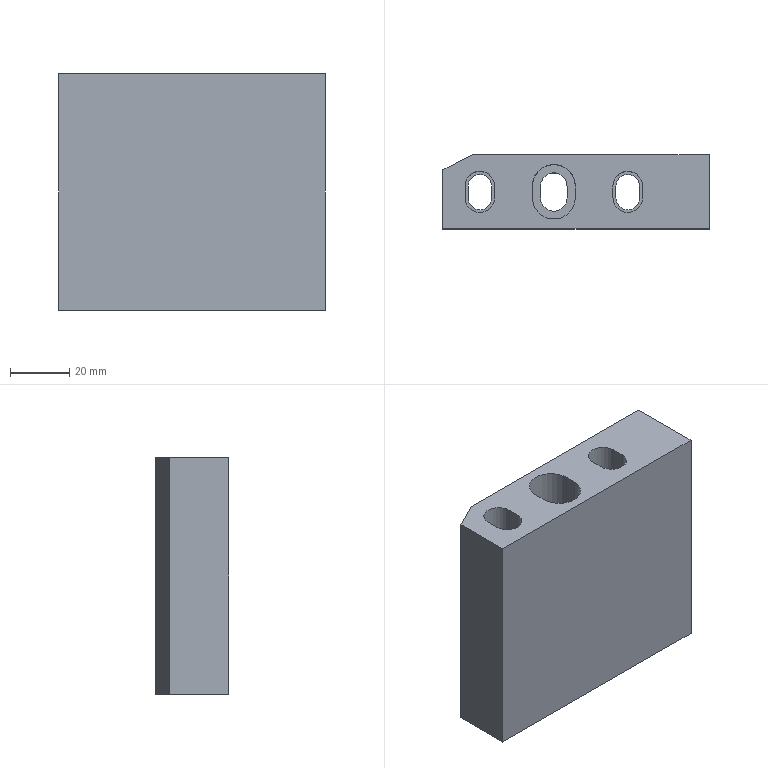Part | STEP file | 1 solid | 34 faces | box 90 x 25 x 80 mm | volume 146448 mm3 | plane 22 | cylinder 12 | commonest cylinder face diameters 8 x4 10 x4 9 x2 14.5 x2
STEP:
#1=CARTESIAN_POINT('',(257.5,-111.,33.));
#2=VERTEX_POINT('',#1);
#3=CARTESIAN_POINT('',(247.5,-111.,33.));
#4=VERTEX_POINT('',#3);
#5=CARTESIAN_POINT('',(252.5,-111.,33.));
#6=DIRECTION('',(0.,0.,-1.));
#7=DIRECTION('',(1.,0.,0.));
#8=AXIS2_PLACEMENT_3D('',#5,#6,#7);
#9=CIRCLE('',#8,5.);
#10=EDGE_CURVE('',#2,#4,#9,.T.);
#11=ORIENTED_EDGE('',*,*,#10,.T.);
#12=CARTESIAN_POINT('',(247.5,-107.,33.));
#13=VERTEX_POINT('',#12);
#14=CARTESIAN_POINT('',(247.5,3.,33.));
#15=DIRECTION('',(0.,1.,0.));
#16=VECTOR('',#15,1.);
#17=LINE('',#14,#16);
#18=EDGE_CURVE('',#4,#13,#17,.T.);
#19=ORIENTED_EDGE('',*,*,#18,.T.);
#20=CARTESIAN_POINT('',(257.5,-107.,33.));
#21=VERTEX_POINT('',#20);
#22=CARTESIAN_POINT('',(252.5,-107.,33.));
#23=DIRECTION('',(0.,0.,-1.));
#24=DIRECTION('',(1.,0.,0.));
#25=AXIS2_PLACEMENT_3D('',#22,#23,#24);
#26=CIRCLE('',#25,5.);
#27=EDGE_CURVE('',#13,#21,#26,.T.);
#28=ORIENTED_EDGE('',*,*,#27,.T.);
#29=CARTESIAN_POINT('',(257.5,3.,33.));
#30=DIRECTION('',(0.,1.,0.));
#31=VECTOR('',#30,1.);
#32=LINE('',#29,#31);
#33=EDGE_CURVE('',#2,#21,#32,.T.);
#34=ORIENTED_EDGE('',*,*,#33,.F.);
#35=EDGE_LOOP('',(#11,#19,#28,#34));
#36=FACE_BOUND('',#35,.T.);
#37=CARTESIAN_POINT('',(307.5,-111.,33.));
#38=VERTEX_POINT('',#37);
#39=CARTESIAN_POINT('',(297.5,-111.,33.));
#40=VERTEX_POINT('',#39);
#41=CARTESIAN_POINT('',(302.5,-111.,33.));
#42=DIRECTION('',(0.,0.,-1.));
#43=DIRECTION('',(1.,0.,0.));
#44=AXIS2_PLACEMENT_3D('',#41,#42,#43);
#45=CIRCLE('',#44,5.);
#46=EDGE_CURVE('',#38,#40,#45,.T.);
#47=ORIENTED_EDGE('',*,*,#46,.T.);
#48=CARTESIAN_POINT('',(297.5,-107.,33.));
#49=VERTEX_POINT('',#48);
#50=CARTESIAN_POINT('',(297.5,3.,33.));
#51=DIRECTION('',(0.,1.,0.));
#52=VECTOR('',#51,1.);
#53=LINE('',#50,#52);
#54=EDGE_CURVE('',#40,#49,#53,.T.);
#55=ORIENTED_EDGE('',*,*,#54,.T.);
#56=CARTESIAN_POINT('',(307.5,-107.,33.));
#57=VERTEX_POINT('',#56);
#58=CARTESIAN_POINT('',(302.5,-107.,33.));
#59=DIRECTION('',(0.,0.,-1.));
#60=DIRECTION('',(1.,0.,0.));
#61=AXIS2_PLACEMENT_3D('',#58,#59,#60);
#62=CIRCLE('',#61,5.);
#63=EDGE_CURVE('',#49,#57,#62,.T.);
#64=ORIENTED_EDGE('',*,*,#63,.T.);
#65=CARTESIAN_POINT('',(307.5,3.,33.));
#66=DIRECTION('',(0.,1.,0.));
#67=VECTOR('',#66,1.);
#68=LINE('',#65,#67);
#69=EDGE_CURVE('',#38,#57,#68,.T.);
#70=ORIENTED_EDGE('',*,*,#69,.F.);
#71=EDGE_LOOP('',(#47,#55,#64,#70));
#72=FACE_BOUND('',#71,.T.);
#73=CARTESIAN_POINT('',(284.75,-111.,33.));
#74=VERTEX_POINT('',#73);
#75=CARTESIAN_POINT('',(270.25,-111.,33.));
#76=VERTEX_POINT('',#75);
#77=CARTESIAN_POINT('',(277.5,-111.,33.));
#78=DIRECTION('',(0.,0.,-1.));
#79=DIRECTION('',(1.,0.,0.));
#80=AXIS2_PLACEMENT_3D('',#77,#78,#79);
#81=CIRCLE('',#80,7.25);
#82=EDGE_CURVE('',#74,#76,#81,.T.);
#83=ORIENTED_EDGE('',*,*,#82,.T.);
#84=CARTESIAN_POINT('',(270.25,-107.,33.));
#85=VERTEX_POINT('',#84);
#86=CARTESIAN_POINT('',(270.25,3.,33.));
#87=DIRECTION('',(0.,1.,0.));
#88=VECTOR('',#87,1.);
#89=LINE('',#86,#88);
#90=EDGE_CURVE('',#76,#85,#89,.T.);
#91=ORIENTED_EDGE('',*,*,#90,.T.);
#92=CARTESIAN_POINT('',(284.75,-107.,33.));
#93=VERTEX_POINT('',#92);
#94=CARTESIAN_POINT('',(277.5,-107.,33.));
#95=DIRECTION('',(0.,0.,-1.));
#96=DIRECTION('',(1.,0.,0.));
#97=AXIS2_PLACEMENT_3D('',#94,#95,#96);
#98=CIRCLE('',#97,7.25);
#99=EDGE_CURVE('',#85,#93,#98,.T.);
#100=ORIENTED_EDGE('',*,*,#99,.T.);
#101=CARTESIAN_POINT('',(284.75,3.,33.));
#102=DIRECTION('',(0.,1.,0.));
#103=VECTOR('',#102,1.);
#104=LINE('',#101,#103);
#105=EDGE_CURVE('',#74,#93,#104,.T.);
#106=ORIENTED_EDGE('',*,*,#105,.F.);
#107=EDGE_LOOP('',(#83,#91,#100,#106));
#108=FACE_BOUND('',#107,.T.);
#109=CARTESIAN_POINT('',(330.,-96.5,33.));
#110=VERTEX_POINT('',#109);
#111=CARTESIAN_POINT('',(250.,-96.5,33.));
#112=VERTEX_POINT('',#111);
#113=CARTESIAN_POINT('',(259.,-96.5,33.));
#114=DIRECTION('',(-1.,0.,0.));
#115=VECTOR('',#114,1.);
#116=LINE('',#113,#115);
#117=EDGE_CURVE('',#110,#112,#116,.T.);
#118=ORIENTED_EDGE('',*,*,#117,.T.);
#119=CARTESIAN_POINT('',(240.,-101.5,33.));
#120=VERTEX_POINT('',#119);
#121=CARTESIAN_POINT('',(240.,-101.5,33.));
#122=DIRECTION('',(-0.8944,-0.4472,0.));
#123=VECTOR('',#122,1.);
#124=LINE('',#121,#123);
#125=EDGE_CURVE('',#112,#120,#124,.T.);
#126=ORIENTED_EDGE('',*,*,#125,.T.);
#127=CARTESIAN_POINT('',(240.,-121.5,33.));
#128=VERTEX_POINT('',#127);
#129=CARTESIAN_POINT('',(240.,-74.5,33.));
#130=DIRECTION('',(0.,1.,0.));
#131=VECTOR('',#130,1.);
#132=LINE('',#129,#131);
#133=EDGE_CURVE('',#128,#120,#132,.T.);
#134=ORIENTED_EDGE('',*,*,#133,.F.);
#135=CARTESIAN_POINT('',(330.,-121.5,33.));
#136=VERTEX_POINT('',#135);
#137=CARTESIAN_POINT('',(259.,-121.5,33.));
#138=DIRECTION('',(-1.,0.,0.));
#139=VECTOR('',#138,1.);
#140=LINE('',#137,#139);
#141=EDGE_CURVE('',#136,#128,#140,.T.);
#142=ORIENTED_EDGE('',*,*,#141,.F.);
#143=CARTESIAN_POINT('',(330.,3.,33.));
#144=DIRECTION('',(0.,1.,0.));
#145=VECTOR('',#144,1.);
#146=LINE('',#143,#145);
#147=EDGE_CURVE('',#136,#110,#146,.T.);
#148=ORIENTED_EDGE('',*,*,#147,.T.);
#149=EDGE_LOOP('',(#118,#126,#134,#142,#148));
#150=FACE_BOUND('',#149,.T.);
#151=CARTESIAN_POINT('',(88.5,3.,33.));
#152=DIRECTION('',(0.,0.,1.));
#153=DIRECTION('',(1.,0.,0.));
#154=AXIS2_PLACEMENT_3D('',#151,#152,#153);
#155=PLANE('',#154);
#156=ADVANCED_FACE('',(#36,#72,#108,#150),#155,.T.);
#157=ORIENTED_EDGE('',*,*,#133,.T.);
#158=CARTESIAN_POINT('',(240.,-101.5,-47.));
#159=VERTEX_POINT('',#158);
#160=CARTESIAN_POINT('',(240.,-101.5,-47.));
#161=DIRECTION('',(0.,0.,-1.));
#162=VECTOR('',#161,1.);
#163=LINE('',#160,#162);
#164=EDGE_CURVE('',#120,#159,#163,.T.);
#165=ORIENTED_EDGE('',*,*,#164,.T.);
#166=CARTESIAN_POINT('',(240.,-121.5,-47.));
#167=VERTEX_POINT('',#166);
#168=CARTESIAN_POINT('',(240.,-74.5,-47.));
#169=DIRECTION('',(0.,1.,0.));
#170=VECTOR('',#169,1.);
#171=LINE('',#168,#170);
#172=EDGE_CURVE('',#167,#159,#171,.T.);
#173=ORIENTED_EDGE('',*,*,#172,.F.);
#174=CARTESIAN_POINT('',(240.,-121.5,-29.347));
#175=DIRECTION('',(0.,0.,-1.));
#176=VECTOR('',#175,1.);
#177=LINE('',#174,#176);
#178=EDGE_CURVE('',#128,#167,#177,.T.);
#179=ORIENTED_EDGE('',*,*,#178,.F.);
#180=EDGE_LOOP('',(#157,#165,#173,#179));
#181=FACE_OUTER_BOUND('',#180,.T.);
#182=CARTESIAN_POINT('',(240.,-74.5,-22.));
#183=DIRECTION('',(1.,0.,0.));
#184=DIRECTION('',(0.,0.,-1.));
#185=AXIS2_PLACEMENT_3D('',#182,#183,#184);
#186=PLANE('',#185);
#187=ADVANCED_FACE('',(#181),#186,.F.);
#188=CARTESIAN_POINT('',(256.5,-107.,-47.));
#189=VERTEX_POINT('',#188);
#190=CARTESIAN_POINT('',(248.5,-107.,-47.));
#191=VERTEX_POINT('',#190);
#192=CARTESIAN_POINT('',(252.5,-107.,-47.));
#193=DIRECTION('',(0.,0.,1.));
#194=DIRECTION('',(1.,0.,0.));
#195=AXIS2_PLACEMENT_3D('',#192,#193,#194);
#196=CIRCLE('',#195,4.);
#197=EDGE_CURVE('',#189,#191,#196,.T.);
#198=ORIENTED_EDGE('',*,*,#197,.T.);
#199=CARTESIAN_POINT('',(248.5,-111.,-47.));
#200=VERTEX_POINT('',#199);
#201=CARTESIAN_POINT('',(248.5,-74.5,-47.));
#202=DIRECTION('',(0.,-1.,0.));
#203=VECTOR('',#202,1.);
#204=LINE('',#201,#203);
#205=EDGE_CURVE('',#191,#200,#204,.T.);
#206=ORIENTED_EDGE('',*,*,#205,.T.);
#207=CARTESIAN_POINT('',(256.5,-111.,-47.));
#208=VERTEX_POINT('',#207);
#209=CARTESIAN_POINT('',(252.5,-111.,-47.));
#210=DIRECTION('',(0.,0.,1.));
#211=DIRECTION('',(1.,0.,0.));
#212=AXIS2_PLACEMENT_3D('',#209,#210,#211);
#213=CIRCLE('',#212,4.);
#214=EDGE_CURVE('',#200,#208,#213,.T.);
#215=ORIENTED_EDGE('',*,*,#214,.T.);
#216=CARTESIAN_POINT('',(256.5,-74.5,-47.));
#217=DIRECTION('',(0.,-1.,0.));
#218=VECTOR('',#217,1.);
#219=LINE('',#216,#218);
#220=EDGE_CURVE('',#189,#208,#219,.T.);
#221=ORIENTED_EDGE('',*,*,#220,.F.);
#222=EDGE_LOOP('',(#198,#206,#215,#221));
#223=FACE_BOUND('',#222,.T.);
#224=CARTESIAN_POINT('',(306.5,-107.,-47.));
#225=VERTEX_POINT('',#224);
#226=CARTESIAN_POINT('',(298.5,-107.,-47.));
#227=VERTEX_POINT('',#226);
#228=CARTESIAN_POINT('',(302.5,-107.,-47.));
#229=DIRECTION('',(0.,0.,1.));
#230=DIRECTION('',(1.,0.,0.));
#231=AXIS2_PLACEMENT_3D('',#228,#229,#230);
#232=CIRCLE('',#231,4.);
#233=EDGE_CURVE('',#225,#227,#232,.T.);
#234=ORIENTED_EDGE('',*,*,#233,.T.);
#235=CARTESIAN_POINT('',(298.5,-111.,-47.));
#236=VERTEX_POINT('',#235);
#237=CARTESIAN_POINT('',(298.5,-74.5,-47.));
#238=DIRECTION('',(0.,-1.,0.));
#239=VECTOR('',#238,1.);
#240=LINE('',#237,#239);
#241=EDGE_CURVE('',#227,#236,#240,.T.);
#242=ORIENTED_EDGE('',*,*,#241,.T.);
#243=CARTESIAN_POINT('',(306.5,-111.,-47.));
#244=VERTEX_POINT('',#243);
#245=CARTESIAN_POINT('',(302.5,-111.,-47.));
#246=DIRECTION('',(0.,0.,1.));
#247=DIRECTION('',(1.,0.,0.));
#248=AXIS2_PLACEMENT_3D('',#245,#246,#247);
#249=CIRCLE('',#248,4.);
#250=EDGE_CURVE('',#236,#244,#249,.T.);
#251=ORIENTED_EDGE('',*,*,#250,.T.);
#252=CARTESIAN_POINT('',(306.5,-74.5,-47.));
#253=DIRECTION('',(0.,-1.,0.));
#254=VECTOR('',#253,1.);
#255=LINE('',#252,#254);
#256=EDGE_CURVE('',#225,#244,#255,.T.);
#257=ORIENTED_EDGE('',*,*,#256,.F.);
#258=EDGE_LOOP('',(#234,#242,#251,#257));
#259=FACE_BOUND('',#258,.T.);
#260=CARTESIAN_POINT('',(282.,-107.,-47.));
#261=VERTEX_POINT('',#260);
#262=CARTESIAN_POINT('',(273.,-107.,-47.));
#263=VERTEX_POINT('',#262);
#264=CARTESIAN_POINT('',(277.5,-107.,-47.));
#265=DIRECTION('',(0.,0.,1.));
#266=DIRECTION('',(1.,0.,0.));
#267=AXIS2_PLACEMENT_3D('',#264,#265,#266);
#268=CIRCLE('',#267,4.5);
#269=EDGE_CURVE('',#261,#263,#268,.T.);
#270=ORIENTED_EDGE('',*,*,#269,.T.);
#271=CARTESIAN_POINT('',(273.,-111.,-47.));
#272=VERTEX_POINT('',#271);
#273=CARTESIAN_POINT('',(273.,-74.5,-47.));
#274=DIRECTION('',(0.,-1.,0.));
#275=VECTOR('',#274,1.);
#276=LINE('',#273,#275);
#277=EDGE_CURVE('',#263,#272,#276,.T.);
#278=ORIENTED_EDGE('',*,*,#277,.T.);
#279=CARTESIAN_POINT('',(282.,-111.,-47.));
#280=VERTEX_POINT('',#279);
#281=CARTESIAN_POINT('',(277.5,-111.,-47.));
#282=DIRECTION('',(0.,0.,1.));
#283=DIRECTION('',(1.,0.,0.));
#284=AXIS2_PLACEMENT_3D('',#281,#282,#283);
#285=CIRCLE('',#284,4.5);
#286=EDGE_CURVE('',#272,#280,#285,.T.);
#287=ORIENTED_EDGE('',*,*,#286,.T.);
#288=CARTESIAN_POINT('',(282.,-74.5,-47.));
#289=DIRECTION('',(0.,-1.,0.));
#290=VECTOR('',#289,1.);
#291=LINE('',#288,#290);
#292=EDGE_CURVE('',#261,#280,#291,.T.);
#293=ORIENTED_EDGE('',*,*,#292,.F.);
#294=EDGE_LOOP('',(#270,#278,#287,#293));
#295=FACE_BOUND('',#294,.T.);
#296=ORIENTED_EDGE('',*,*,#172,.T.);
#297=CARTESIAN_POINT('',(250.,-96.5,-47.));
#298=VERTEX_POINT('',#297);
#299=CARTESIAN_POINT('',(240.,-101.5,-47.));
#300=DIRECTION('',(0.8944,0.4472,0.));
#301=VECTOR('',#300,1.);
#302=LINE('',#299,#301);
#303=EDGE_CURVE('',#159,#298,#302,.T.);
#304=ORIENTED_EDGE('',*,*,#303,.T.);
#305=CARTESIAN_POINT('',(330.,-96.5,-47.));
#306=VERTEX_POINT('',#305);
#307=CARTESIAN_POINT('',(259.,-96.5,-47.));
#308=DIRECTION('',(1.,0.,0.));
#309=VECTOR('',#308,1.);
#310=LINE('',#307,#309);
#311=EDGE_CURVE('',#298,#306,#310,.T.);
#312=ORIENTED_EDGE('',*,*,#311,.T.);
#313=CARTESIAN_POINT('',(330.,-121.5,-47.));
#314=VERTEX_POINT('',#313);
#315=CARTESIAN_POINT('',(330.,-74.5,-47.));
#316=DIRECTION('',(0.,1.,0.));
#317=VECTOR('',#316,1.);
#318=LINE('',#315,#317);
#319=EDGE_CURVE('',#314,#306,#318,.T.);
#320=ORIENTED_EDGE('',*,*,#319,.F.);
#321=CARTESIAN_POINT('',(259.,-121.5,-47.));
#322=DIRECTION('',(1.,0.,0.));
#323=VECTOR('',#322,1.);
#324=LINE('',#321,#323);
#325=EDGE_CURVE('',#167,#314,#324,.T.);
#326=ORIENTED_EDGE('',*,*,#325,.F.);
#327=EDGE_LOOP('',(#296,#304,#312,#320,#326));
#328=FACE_BOUND('',#327,.T.);
#329=CARTESIAN_POINT('',(259.,-74.5,-47.));
#330=DIRECTION('',(0.,0.,1.));
#331=DIRECTION('',(1.,0.,0.));
#332=AXIS2_PLACEMENT_3D('',#329,#330,#331);
#333=PLANE('',#332);
#334=ADVANCED_FACE('',(#223,#259,#295,#328),#333,.F.);
#335=CARTESIAN_POINT('',(330.,-121.5,-29.347));
#336=DIRECTION('',(0.,0.,-1.));
#337=VECTOR('',#336,1.);
#338=LINE('',#335,#337);
#339=EDGE_CURVE('',#136,#314,#338,.T.);
#340=ORIENTED_EDGE('',*,*,#339,.T.);
#341=ORIENTED_EDGE('',*,*,#319,.T.);
#342=CARTESIAN_POINT('',(330.,-96.5,-29.347));
#343=DIRECTION('',(0.,0.,-1.));
#344=VECTOR('',#343,1.);
#345=LINE('',#342,#344);
#346=EDGE_CURVE('',#110,#306,#345,.T.);
#347=ORIENTED_EDGE('',*,*,#346,.F.);
#348=ORIENTED_EDGE('',*,*,#147,.F.);
#349=EDGE_LOOP('',(#340,#341,#347,#348));
#350=FACE_OUTER_BOUND('',#349,.T.);
#351=CARTESIAN_POINT('',(330.,-74.5,-29.347));
#352=DIRECTION('',(-1.,0.,0.));
#353=DIRECTION('',(0.,0.,1.));
#354=AXIS2_PLACEMENT_3D('',#351,#352,#353);
#355=PLANE('',#354);
#356=ADVANCED_FACE('',(#350),#355,.F.);
#357=ORIENTED_EDGE('',*,*,#311,.F.);
#358=CARTESIAN_POINT('',(250.,-96.5,33.));
#359=DIRECTION('',(0.,0.,1.));
#360=VECTOR('',#359,1.);
#361=LINE('',#358,#360);
#362=EDGE_CURVE('',#298,#112,#361,.T.);
#363=ORIENTED_EDGE('',*,*,#362,.T.);
#364=ORIENTED_EDGE('',*,*,#117,.F.);
#365=ORIENTED_EDGE('',*,*,#346,.T.);
#366=EDGE_LOOP('',(#357,#363,#364,#365));
#367=FACE_OUTER_BOUND('',#366,.T.);
#368=CARTESIAN_POINT('',(259.,-96.5,-29.347));
#369=DIRECTION('',(0.,1.,0.));
#370=DIRECTION('',(0.,0.,1.));
#371=AXIS2_PLACEMENT_3D('',#368,#369,#370);
#372=PLANE('',#371);
#373=ADVANCED_FACE('',(#367),#372,.T.);
#374=ORIENTED_EDGE('',*,*,#325,.T.);
#375=ORIENTED_EDGE('',*,*,#339,.F.);
#376=ORIENTED_EDGE('',*,*,#141,.T.);
#377=ORIENTED_EDGE('',*,*,#178,.T.);
#378=EDGE_LOOP('',(#374,#375,#376,#377));
#379=FACE_OUTER_BOUND('',#378,.T.);
#380=CARTESIAN_POINT('',(259.,-121.5,-29.347));
#381=DIRECTION('',(0.,1.,0.));
#382=DIRECTION('',(0.,0.,1.));
#383=AXIS2_PLACEMENT_3D('',#380,#381,#382);
#384=PLANE('',#383);
#385=ADVANCED_FACE('',(#379),#384,.F.);
#386=ORIENTED_EDGE('',*,*,#125,.F.);
#387=ORIENTED_EDGE('',*,*,#362,.F.);
#388=ORIENTED_EDGE('',*,*,#303,.F.);
#389=ORIENTED_EDGE('',*,*,#164,.F.);
#390=EDGE_LOOP('',(#386,#387,#388,#389));
#391=FACE_OUTER_BOUND('',#390,.T.);
#392=CARTESIAN_POINT('',(240.,-101.5,-22.));
#393=DIRECTION('',(-0.4472,0.8944,0.));
#394=DIRECTION('',(0.,0.,1.));
#395=AXIS2_PLACEMENT_3D('',#392,#393,#394);
#396=PLANE('',#395);
#397=ADVANCED_FACE('',(#391),#396,.T.);
#398=CARTESIAN_POINT('',(270.25,-111.,-22.));
#399=VERTEX_POINT('',#398);
#400=CARTESIAN_POINT('',(270.25,-111.,-22.));
#401=DIRECTION('',(0.,0.,-1.));
#402=VECTOR('',#401,1.);
#403=LINE('',#400,#402);
#404=EDGE_CURVE('',#76,#399,#403,.T.);
#405=ORIENTED_EDGE('',*,*,#404,.T.);
#406=CARTESIAN_POINT('',(270.25,-107.,-22.));
#407=VERTEX_POINT('',#406);
#408=CARTESIAN_POINT('',(270.25,-107.,-22.));
#409=DIRECTION('',(0.,1.,0.));
#410=VECTOR('',#409,1.);
#411=LINE('',#408,#410);
#412=EDGE_CURVE('',#399,#407,#411,.T.);
#413=ORIENTED_EDGE('',*,*,#412,.T.);
#414=CARTESIAN_POINT('',(270.25,-107.,-22.));
#415=DIRECTION('',(0.,0.,-1.));
#416=VECTOR('',#415,1.);
#417=LINE('',#414,#416);
#418=EDGE_CURVE('',#85,#407,#417,.T.);
#419=ORIENTED_EDGE('',*,*,#418,.F.);
#420=ORIENTED_EDGE('',*,*,#90,.F.);
#421=EDGE_LOOP('',(#405,#413,#419,#420));
#422=FACE_OUTER_BOUND('',#421,.T.);
#423=CARTESIAN_POINT('',(270.25,-107.,-22.));
#424=DIRECTION('',(-1.,0.,0.));
#425=DIRECTION('',(0.,0.,1.));
#426=AXIS2_PLACEMENT_3D('',#423,#424,#425);
#427=PLANE('',#426);
#428=ADVANCED_FACE('',(#422),#427,.F.);
#429=CARTESIAN_POINT('',(284.75,-111.,-22.));
#430=VERTEX_POINT('',#429);
#431=CARTESIAN_POINT('',(284.75,-111.,-22.));
#432=DIRECTION('',(0.,0.,-1.));
#433=VECTOR('',#432,1.);
#434=LINE('',#431,#433);
#435=EDGE_CURVE('',#74,#430,#434,.T.);
#436=ORIENTED_EDGE('',*,*,#435,.T.);
#437=CARTESIAN_POINT('',(277.5,-111.,-22.));
#438=DIRECTION('',(0.,0.,-1.));
#439=DIRECTION('',(1.,0.,0.));
#440=AXIS2_PLACEMENT_3D('',#437,#438,#439);
#441=CIRCLE('',#440,7.25);
#442=EDGE_CURVE('',#430,#399,#441,.T.);
#443=ORIENTED_EDGE('',*,*,#442,.T.);
#444=ORIENTED_EDGE('',*,*,#404,.F.);
#445=ORIENTED_EDGE('',*,*,#82,.F.);
#446=EDGE_LOOP('',(#436,#443,#444,#445));
#447=FACE_OUTER_BOUND('',#446,.T.);
#448=CARTESIAN_POINT('',(277.5,-111.,-22.));
#449=DIRECTION('',(0.,0.,1.));
#450=DIRECTION('',(1.,0.,0.));
#451=AXIS2_PLACEMENT_3D('',#448,#449,#450);
#452=CYLINDRICAL_SURFACE('',#451,7.25);
#453=ADVANCED_FACE('',(#447),#452,.F.);
#454=ORIENTED_EDGE('',*,*,#105,.T.);
#455=CARTESIAN_POINT('',(284.75,-107.,-22.));
#456=VERTEX_POINT('',#455);
#457=CARTESIAN_POINT('',(284.75,-107.,-22.));
#458=DIRECTION('',(0.,0.,-1.));
#459=VECTOR('',#458,1.);
#460=LINE('',#457,#459);
#461=EDGE_CURVE('',#93,#456,#460,.T.);
#462=ORIENTED_EDGE('',*,*,#461,.T.);
#463=CARTESIAN_POINT('',(284.75,-107.,-22.));
#464=DIRECTION('',(0.,1.,0.));
#465=VECTOR('',#464,1.);
#466=LINE('',#463,#465);
#467=EDGE_CURVE('',#430,#456,#466,.T.);
#468=ORIENTED_EDGE('',*,*,#467,.F.);
#469=ORIENTED_EDGE('',*,*,#435,.F.);
#470=EDGE_LOOP('',(#454,#462,#468,#469));
#471=FACE_OUTER_BOUND('',#470,.T.);
#472=CARTESIAN_POINT('',(284.75,-107.,-22.));
#473=DIRECTION('',(-1.,0.,0.));
#474=DIRECTION('',(0.,0.,1.));
#475=AXIS2_PLACEMENT_3D('',#472,#473,#474);
#476=PLANE('',#475);
#477=ADVANCED_FACE('',(#471),#476,.T.);
#478=ORIENTED_EDGE('',*,*,#418,.T.);
#479=CARTESIAN_POINT('',(277.5,-107.,-22.));
#480=DIRECTION('',(0.,0.,-1.));
#481=DIRECTION('',(1.,0.,0.));
#482=AXIS2_PLACEMENT_3D('',#479,#480,#481);
#483=CIRCLE('',#482,7.25);
#484=EDGE_CURVE('',#407,#456,#483,.T.);
#485=ORIENTED_EDGE('',*,*,#484,.T.);
#486=ORIENTED_EDGE('',*,*,#461,.F.);
#487=ORIENTED_EDGE('',*,*,#99,.F.);
#488=EDGE_LOOP('',(#478,#485,#486,#487));
#489=FACE_OUTER_BOUND('',#488,.T.);
#490=CARTESIAN_POINT('',(277.5,-107.,-22.));
#491=DIRECTION('',(0.,0.,1.));
#492=DIRECTION('',(1.,0.,0.));
#493=AXIS2_PLACEMENT_3D('',#490,#491,#492);
#494=CYLINDRICAL_SURFACE('',#493,7.25);
#495=ADVANCED_FACE('',(#489),#494,.F.);
#496=CARTESIAN_POINT('',(273.,-107.,-22.));
#497=VERTEX_POINT('',#496);
#498=CARTESIAN_POINT('',(273.,-107.,-48.));
#499=DIRECTION('',(0.,0.,-1.));
#500=VECTOR('',#499,1.);
#501=LINE('',#498,#500);
#502=EDGE_CURVE('',#497,#263,#501,.T.);
#503=ORIENTED_EDGE('',*,*,#502,.F.);
#504=CARTESIAN_POINT('',(273.,-111.,-22.));
#505=VERTEX_POINT('',#504);
#506=CARTESIAN_POINT('',(273.,-107.,-22.));
#507=DIRECTION('',(0.,-1.,0.));
#508=VECTOR('',#507,1.);
#509=LINE('',#506,#508);
#510=EDGE_CURVE('',#497,#505,#509,.T.);
#511=ORIENTED_EDGE('',*,*,#510,.T.);
#512=CARTESIAN_POINT('',(273.,-111.,-48.));
#513=DIRECTION('',(0.,0.,-1.));
#514=VECTOR('',#513,1.);
#515=LINE('',#512,#514);
#516=EDGE_CURVE('',#505,#272,#515,.T.);
#517=ORIENTED_EDGE('',*,*,#516,.T.);
#518=ORIENTED_EDGE('',*,*,#277,.F.);
#519=EDGE_LOOP('',(#503,#511,#517,#518));
#520=FACE_OUTER_BOUND('',#519,.T.);
#521=CARTESIAN_POINT('',(273.,-107.,-48.));
#522=DIRECTION('',(-1.,0.,0.));
#523=DIRECTION('',(0.,0.,1.));
#524=AXIS2_PLACEMENT_3D('',#521,#522,#523);
#525=PLANE('',#524);
#526=ADVANCED_FACE('',(#520),#525,.F.);
#527=ORIENTED_EDGE('',*,*,#516,.F.);
#528=CARTESIAN_POINT('',(282.,-111.,-22.));
#529=VERTEX_POINT('',#528);
#530=CARTESIAN_POINT('',(277.5,-111.,-22.));
#531=DIRECTION('',(0.,0.,1.));
#532=DIRECTION('',(1.,0.,0.));
#533=AXIS2_PLACEMENT_3D('',#530,#531,#532);
#534=CIRCLE('',#533,4.5);
#535=EDGE_CURVE('',#505,#529,#534,.T.);
#536=ORIENTED_EDGE('',*,*,#535,.T.);
#537=CARTESIAN_POINT('',(282.,-111.,-48.));
#538=DIRECTION('',(0.,0.,-1.));
#539=VECTOR('',#538,1.);
#540=LINE('',#537,#539);
#541=EDGE_CURVE('',#529,#280,#540,.T.);
#542=ORIENTED_EDGE('',*,*,#541,.T.);
#543=ORIENTED_EDGE('',*,*,#286,.F.);
#544=EDGE_LOOP('',(#527,#536,#542,#543));
#545=FACE_OUTER_BOUND('',#544,.T.);
#546=CARTESIAN_POINT('',(277.5,-111.,-48.));
#547=DIRECTION('',(0.,0.,1.));
#548=DIRECTION('',(1.,0.,0.));
#549=AXIS2_PLACEMENT_3D('',#546,#547,#548);
#550=CYLINDRICAL_SURFACE('',#549,4.5);
#551=ADVANCED_FACE('',(#545),#550,.F.);
#552=ORIENTED_EDGE('',*,*,#292,.T.);
#553=ORIENTED_EDGE('',*,*,#541,.F.);
#554=CARTESIAN_POINT('',(282.,-107.,-22.));
#555=VERTEX_POINT('',#554);
#556=CARTESIAN_POINT('',(282.,-107.,-22.));
#557=DIRECTION('',(0.,-1.,0.));
#558=VECTOR('',#557,1.);
#559=LINE('',#556,#558);
#560=EDGE_CURVE('',#555,#529,#559,.T.);
#561=ORIENTED_EDGE('',*,*,#560,.F.);
#562=CARTESIAN_POINT('',(282.,-107.,-48.));
#563=DIRECTION('',(0.,0.,-1.));
#564=VECTOR('',#563,1.);
#565=LINE('',#562,#564);
#566=EDGE_CURVE('',#555,#261,#565,.T.);
#567=ORIENTED_EDGE('',*,*,#566,.T.);
#568=EDGE_LOOP('',(#552,#553,#561,#567));
#569=FACE_OUTER_BOUND('',#568,.T.);
#570=CARTESIAN_POINT('',(282.,-107.,-48.));
#571=DIRECTION('',(-1.,0.,0.));
#572=DIRECTION('',(0.,0.,1.));
#573=AXIS2_PLACEMENT_3D('',#570,#571,#572);
#574=PLANE('',#573);
#575=ADVANCED_FACE('',(#569),#574,.T.);
#576=ORIENTED_EDGE('',*,*,#566,.F.);
#577=CARTESIAN_POINT('',(277.5,-107.,-22.));
#578=DIRECTION('',(0.,0.,1.));
#579=DIRECTION('',(1.,0.,0.));
#580=AXIS2_PLACEMENT_3D('',#577,#578,#579);
#581=CIRCLE('',#580,4.5);
#582=EDGE_CURVE('',#555,#497,#581,.T.);
#583=ORIENTED_EDGE('',*,*,#582,.T.);
#584=ORIENTED_EDGE('',*,*,#502,.T.);
#585=ORIENTED_EDGE('',*,*,#269,.F.);
#586=EDGE_LOOP('',(#576,#583,#584,#585));
#587=FACE_OUTER_BOUND('',#586,.T.);
#588=CARTESIAN_POINT('',(277.5,-107.,-48.));
#589=DIRECTION('',(0.,0.,1.));
#590=DIRECTION('',(1.,0.,0.));
#591=AXIS2_PLACEMENT_3D('',#588,#589,#590);
#592=CYLINDRICAL_SURFACE('',#591,4.5);
#593=ADVANCED_FACE('',(#587),#592,.F.);
#594=ORIENTED_EDGE('',*,*,#510,.F.);
#595=ORIENTED_EDGE('',*,*,#582,.F.);
#596=ORIENTED_EDGE('',*,*,#560,.T.);
#597=ORIENTED_EDGE('',*,*,#535,.F.);
#598=EDGE_LOOP('',(#594,#595,#596,#597));
#599=FACE_BOUND('',#598,.T.);
#600=ORIENTED_EDGE('',*,*,#412,.F.);
#601=ORIENTED_EDGE('',*,*,#442,.F.);
#602=ORIENTED_EDGE('',*,*,#467,.T.);
#603=ORIENTED_EDGE('',*,*,#484,.F.);
#604=EDGE_LOOP('',(#600,#601,#602,#603));
#605=FACE_BOUND('',#604,.T.);
#606=CARTESIAN_POINT('',(277.5,-111.,-22.));
#607=DIRECTION('',(0.,0.,1.));
#608=DIRECTION('',(1.,0.,0.));
#609=AXIS2_PLACEMENT_3D('',#606,#607,#608);
#610=PLANE('',#609);
#611=ADVANCED_FACE('',(#599,#605),#610,.T.);
#612=CARTESIAN_POINT('',(297.5,-111.,-17.));
#613=VERTEX_POINT('',#612);
#614=CARTESIAN_POINT('',(297.5,-111.,-17.));
#615=DIRECTION('',(0.,0.,-1.));
#616=VECTOR('',#615,1.);
#617=LINE('',#614,#616);
#618=EDGE_CURVE('',#40,#613,#617,.T.);
#619=ORIENTED_EDGE('',*,*,#618,.T.);
#620=CARTESIAN_POINT('',(297.5,-107.,-17.));
#621=VERTEX_POINT('',#620);
#622=CARTESIAN_POINT('',(297.5,-107.,-17.));
#623=DIRECTION('',(0.,1.,0.));
#624=VECTOR('',#623,1.);
#625=LINE('',#622,#624);
#626=EDGE_CURVE('',#613,#621,#625,.T.);
#627=ORIENTED_EDGE('',*,*,#626,.T.);
#628=CARTESIAN_POINT('',(297.5,-107.,-17.));
#629=DIRECTION('',(0.,0.,-1.));
#630=VECTOR('',#629,1.);
#631=LINE('',#628,#630);
#632=EDGE_CURVE('',#49,#621,#631,.T.);
#633=ORIENTED_EDGE('',*,*,#632,.F.);
#634=ORIENTED_EDGE('',*,*,#54,.F.);
#635=EDGE_LOOP('',(#619,#627,#633,#634));
#636=FACE_OUTER_BOUND('',#635,.T.);
#637=CARTESIAN_POINT('',(297.5,-107.,-17.));
#638=DIRECTION('',(-1.,0.,0.));
#639=DIRECTION('',(0.,0.,1.));
#640=AXIS2_PLACEMENT_3D('',#637,#638,#639);
#641=PLANE('',#640);
#642=ADVANCED_FACE('',(#636),#641,.F.);
#643=CARTESIAN_POINT('',(307.5,-111.,-17.));
#644=VERTEX_POINT('',#643);
#645=CARTESIAN_POINT('',(307.5,-111.,-17.));
#646=DIRECTION('',(0.,0.,-1.));
#647=VECTOR('',#646,1.);
#648=LINE('',#645,#647);
#649=EDGE_CURVE('',#38,#644,#648,.T.);
#650=ORIENTED_EDGE('',*,*,#649,.T.);
#651=CARTESIAN_POINT('',(302.5,-111.,-17.));
#652=DIRECTION('',(0.,0.,-1.));
#653=DIRECTION('',(1.,0.,0.));
#654=AXIS2_PLACEMENT_3D('',#651,#652,#653);
#655=CIRCLE('',#654,5.);
#656=EDGE_CURVE('',#644,#613,#655,.T.);
#657=ORIENTED_EDGE('',*,*,#656,.T.);
#658=ORIENTED_EDGE('',*,*,#618,.F.);
#659=ORIENTED_EDGE('',*,*,#46,.F.);
#660=EDGE_LOOP('',(#650,#657,#658,#659));
#661=FACE_OUTER_BOUND('',#660,.T.);
#662=CARTESIAN_POINT('',(302.5,-111.,-17.));
#663=DIRECTION('',(0.,0.,1.));
#664=DIRECTION('',(1.,0.,0.));
#665=AXIS2_PLACEMENT_3D('',#662,#663,#664);
#666=CYLINDRICAL_SURFACE('',#665,5.);
#667=ADVANCED_FACE('',(#661),#666,.F.);
#668=ORIENTED_EDGE('',*,*,#69,.T.);
#669=CARTESIAN_POINT('',(307.5,-107.,-17.));
#670=VERTEX_POINT('',#669);
#671=CARTESIAN_POINT('',(307.5,-107.,-17.));
#672=DIRECTION('',(0.,0.,-1.));
#673=VECTOR('',#672,1.);
#674=LINE('',#671,#673);
#675=EDGE_CURVE('',#57,#670,#674,.T.);
#676=ORIENTED_EDGE('',*,*,#675,.T.);
#677=CARTESIAN_POINT('',(307.5,-107.,-17.));
#678=DIRECTION('',(0.,1.,0.));
#679=VECTOR('',#678,1.);
#680=LINE('',#677,#679);
#681=EDGE_CURVE('',#644,#670,#680,.T.);
#682=ORIENTED_EDGE('',*,*,#681,.F.);
#683=ORIENTED_EDGE('',*,*,#649,.F.);
#684=EDGE_LOOP('',(#668,#676,#682,#683));
#685=FACE_OUTER_BOUND('',#684,.T.);
#686=CARTESIAN_POINT('',(307.5,-107.,-17.));
#687=DIRECTION('',(-1.,0.,0.));
#688=DIRECTION('',(0.,0.,1.));
#689=AXIS2_PLACEMENT_3D('',#686,#687,#688);
#690=PLANE('',#689);
#691=ADVANCED_FACE('',(#685),#690,.T.);
#692=ORIENTED_EDGE('',*,*,#632,.T.);
#693=CARTESIAN_POINT('',(302.5,-107.,-17.));
#694=DIRECTION('',(0.,0.,-1.));
#695=DIRECTION('',(1.,0.,0.));
#696=AXIS2_PLACEMENT_3D('',#693,#694,#695);
#697=CIRCLE('',#696,5.);
#698=EDGE_CURVE('',#621,#670,#697,.T.);
#699=ORIENTED_EDGE('',*,*,#698,.T.);
#700=ORIENTED_EDGE('',*,*,#675,.F.);
#701=ORIENTED_EDGE('',*,*,#63,.F.);
#702=EDGE_LOOP('',(#692,#699,#700,#701));
#703=FACE_OUTER_BOUND('',#702,.T.);
#704=CARTESIAN_POINT('',(302.5,-107.,-17.));
#705=DIRECTION('',(0.,0.,1.));
#706=DIRECTION('',(1.,0.,0.));
#707=AXIS2_PLACEMENT_3D('',#704,#705,#706);
#708=CYLINDRICAL_SURFACE('',#707,5.);
#709=ADVANCED_FACE('',(#703),#708,.F.);
#710=CARTESIAN_POINT('',(298.5,-107.,-17.));
#711=VERTEX_POINT('',#710);
#712=CARTESIAN_POINT('',(298.5,-107.,-48.));
#713=DIRECTION('',(0.,0.,-1.));
#714=VECTOR('',#713,1.);
#715=LINE('',#712,#714);
#716=EDGE_CURVE('',#711,#227,#715,.T.);
#717=ORIENTED_EDGE('',*,*,#716,.F.);
#718=CARTESIAN_POINT('',(298.5,-111.,-17.));
#719=VERTEX_POINT('',#718);
#720=CARTESIAN_POINT('',(298.5,-107.,-17.));
#721=DIRECTION('',(0.,-1.,0.));
#722=VECTOR('',#721,1.);
#723=LINE('',#720,#722);
#724=EDGE_CURVE('',#711,#719,#723,.T.);
#725=ORIENTED_EDGE('',*,*,#724,.T.);
#726=CARTESIAN_POINT('',(298.5,-111.,-48.));
#727=DIRECTION('',(0.,0.,-1.));
#728=VECTOR('',#727,1.);
#729=LINE('',#726,#728);
#730=EDGE_CURVE('',#719,#236,#729,.T.);
#731=ORIENTED_EDGE('',*,*,#730,.T.);
#732=ORIENTED_EDGE('',*,*,#241,.F.);
#733=EDGE_LOOP('',(#717,#725,#731,#732));
#734=FACE_OUTER_BOUND('',#733,.T.);
#735=CARTESIAN_POINT('',(298.5,-107.,-48.));
#736=DIRECTION('',(-1.,0.,0.));
#737=DIRECTION('',(0.,0.,1.));
#738=AXIS2_PLACEMENT_3D('',#735,#736,#737);
#739=PLANE('',#738);
#740=ADVANCED_FACE('',(#734),#739,.F.);
#741=ORIENTED_EDGE('',*,*,#730,.F.);
#742=CARTESIAN_POINT('',(306.5,-111.,-17.));
#743=VERTEX_POINT('',#742);
#744=CARTESIAN_POINT('',(302.5,-111.,-17.));
#745=DIRECTION('',(0.,0.,1.));
#746=DIRECTION('',(1.,0.,0.));
#747=AXIS2_PLACEMENT_3D('',#744,#745,#746);
#748=CIRCLE('',#747,4.);
#749=EDGE_CURVE('',#719,#743,#748,.T.);
#750=ORIENTED_EDGE('',*,*,#749,.T.);
#751=CARTESIAN_POINT('',(306.5,-111.,-48.));
#752=DIRECTION('',(0.,0.,-1.));
#753=VECTOR('',#752,1.);
#754=LINE('',#751,#753);
#755=EDGE_CURVE('',#743,#244,#754,.T.);
#756=ORIENTED_EDGE('',*,*,#755,.T.);
#757=ORIENTED_EDGE('',*,*,#250,.F.);
#758=EDGE_LOOP('',(#741,#750,#756,#757));
#759=FACE_OUTER_BOUND('',#758,.T.);
#760=CARTESIAN_POINT('',(302.5,-111.,-48.));
#761=DIRECTION('',(0.,0.,1.));
#762=DIRECTION('',(1.,0.,0.));
#763=AXIS2_PLACEMENT_3D('',#760,#761,#762);
#764=CYLINDRICAL_SURFACE('',#763,4.);
#765=ADVANCED_FACE('',(#759),#764,.F.);
#766=ORIENTED_EDGE('',*,*,#256,.T.);
#767=ORIENTED_EDGE('',*,*,#755,.F.);
#768=CARTESIAN_POINT('',(306.5,-107.,-17.));
#769=VERTEX_POINT('',#768);
#770=CARTESIAN_POINT('',(306.5,-107.,-17.));
#771=DIRECTION('',(0.,-1.,0.));
#772=VECTOR('',#771,1.);
#773=LINE('',#770,#772);
#774=EDGE_CURVE('',#769,#743,#773,.T.);
#775=ORIENTED_EDGE('',*,*,#774,.F.);
#776=CARTESIAN_POINT('',(306.5,-107.,-48.));
#777=DIRECTION('',(0.,0.,-1.));
#778=VECTOR('',#777,1.);
#779=LINE('',#776,#778);
#780=EDGE_CURVE('',#769,#225,#779,.T.);
#781=ORIENTED_EDGE('',*,*,#780,.T.);
#782=EDGE_LOOP('',(#766,#767,#775,#781));
#783=FACE_OUTER_BOUND('',#782,.T.);
#784=CARTESIAN_POINT('',(306.5,-107.,-48.));
#785=DIRECTION('',(-1.,0.,0.));
#786=DIRECTION('',(0.,0.,1.));
#787=AXIS2_PLACEMENT_3D('',#784,#785,#786);
#788=PLANE('',#787);
#789=ADVANCED_FACE('',(#783),#788,.T.);
#790=ORIENTED_EDGE('',*,*,#780,.F.);
#791=CARTESIAN_POINT('',(302.5,-107.,-17.));
#792=DIRECTION('',(0.,0.,1.));
#793=DIRECTION('',(1.,0.,0.));
#794=AXIS2_PLACEMENT_3D('',#791,#792,#793);
#795=CIRCLE('',#794,4.);
#796=EDGE_CURVE('',#769,#711,#795,.T.);
#797=ORIENTED_EDGE('',*,*,#796,.T.);
#798=ORIENTED_EDGE('',*,*,#716,.T.);
#799=ORIENTED_EDGE('',*,*,#233,.F.);
#800=EDGE_LOOP('',(#790,#797,#798,#799));
#801=FACE_OUTER_BOUND('',#800,.T.);
#802=CARTESIAN_POINT('',(302.5,-107.,-48.));
#803=DIRECTION('',(0.,0.,1.));
#804=DIRECTION('',(1.,0.,0.));
#805=AXIS2_PLACEMENT_3D('',#802,#803,#804);
#806=CYLINDRICAL_SURFACE('',#805,4.);
#807=ADVANCED_FACE('',(#801),#806,.F.);
#808=ORIENTED_EDGE('',*,*,#724,.F.);
#809=ORIENTED_EDGE('',*,*,#796,.F.);
#810=ORIENTED_EDGE('',*,*,#774,.T.);
#811=ORIENTED_EDGE('',*,*,#749,.F.);
#812=EDGE_LOOP('',(#808,#809,#810,#811));
#813=FACE_BOUND('',#812,.T.);
#814=ORIENTED_EDGE('',*,*,#626,.F.);
#815=ORIENTED_EDGE('',*,*,#656,.F.);
#816=ORIENTED_EDGE('',*,*,#681,.T.);
#817=ORIENTED_EDGE('',*,*,#698,.F.);
#818=EDGE_LOOP('',(#814,#815,#816,#817));
#819=FACE_BOUND('',#818,.T.);
#820=CARTESIAN_POINT('',(302.5,-111.,-17.));
#821=DIRECTION('',(0.,0.,1.));
#822=DIRECTION('',(1.,0.,0.));
#823=AXIS2_PLACEMENT_3D('',#820,#821,#822);
#824=PLANE('',#823);
#825=ADVANCED_FACE('',(#813,#819),#824,.T.);
#826=CARTESIAN_POINT('',(247.5,-111.,-17.));
#827=VERTEX_POINT('',#826);
#828=CARTESIAN_POINT('',(247.5,-111.,-17.));
#829=DIRECTION('',(0.,0.,-1.));
#830=VECTOR('',#829,1.);
#831=LINE('',#828,#830);
#832=EDGE_CURVE('',#4,#827,#831,.T.);
#833=ORIENTED_EDGE('',*,*,#832,.T.);
#834=CARTESIAN_POINT('',(247.5,-107.,-17.));
#835=VERTEX_POINT('',#834);
#836=CARTESIAN_POINT('',(247.5,-107.,-17.));
#837=DIRECTION('',(0.,1.,0.));
#838=VECTOR('',#837,1.);
#839=LINE('',#836,#838);
#840=EDGE_CURVE('',#827,#835,#839,.T.);
#841=ORIENTED_EDGE('',*,*,#840,.T.);
#842=CARTESIAN_POINT('',(247.5,-107.,-17.));
#843=DIRECTION('',(0.,0.,-1.));
#844=VECTOR('',#843,1.);
#845=LINE('',#842,#844);
#846=EDGE_CURVE('',#13,#835,#845,.T.);
#847=ORIENTED_EDGE('',*,*,#846,.F.);
#848=ORIENTED_EDGE('',*,*,#18,.F.);
#849=EDGE_LOOP('',(#833,#841,#847,#848));
#850=FACE_OUTER_BOUND('',#849,.T.);
#851=CARTESIAN_POINT('',(247.5,-107.,-17.));
#852=DIRECTION('',(-1.,0.,0.));
#853=DIRECTION('',(0.,0.,1.));
#854=AXIS2_PLACEMENT_3D('',#851,#852,#853);
#855=PLANE('',#854);
#856=ADVANCED_FACE('',(#850),#855,.F.);
#857=CARTESIAN_POINT('',(257.5,-111.,-17.));
#858=VERTEX_POINT('',#857);
#859=CARTESIAN_POINT('',(257.5,-111.,-17.));
#860=DIRECTION('',(0.,0.,-1.));
#861=VECTOR('',#860,1.);
#862=LINE('',#859,#861);
#863=EDGE_CURVE('',#2,#858,#862,.T.);
#864=ORIENTED_EDGE('',*,*,#863,.T.);
#865=CARTESIAN_POINT('',(252.5,-111.,-17.));
#866=DIRECTION('',(0.,0.,-1.));
#867=DIRECTION('',(1.,0.,0.));
#868=AXIS2_PLACEMENT_3D('',#865,#866,#867);
#869=CIRCLE('',#868,5.);
#870=EDGE_CURVE('',#858,#827,#869,.T.);
#871=ORIENTED_EDGE('',*,*,#870,.T.);
#872=ORIENTED_EDGE('',*,*,#832,.F.);
#873=ORIENTED_EDGE('',*,*,#10,.F.);
#874=EDGE_LOOP('',(#864,#871,#872,#873));
#875=FACE_OUTER_BOUND('',#874,.T.);
#876=CARTESIAN_POINT('',(252.5,-111.,-17.));
#877=DIRECTION('',(0.,0.,1.));
#878=DIRECTION('',(1.,0.,0.));
#879=AXIS2_PLACEMENT_3D('',#876,#877,#878);
#880=CYLINDRICAL_SURFACE('',#879,5.);
#881=ADVANCED_FACE('',(#875),#880,.F.);
#882=ORIENTED_EDGE('',*,*,#33,.T.);
#883=CARTESIAN_POINT('',(257.5,-107.,-17.));
#884=VERTEX_POINT('',#883);
#885=CARTESIAN_POINT('',(257.5,-107.,-17.));
#886=DIRECTION('',(0.,0.,-1.));
#887=VECTOR('',#886,1.);
#888=LINE('',#885,#887);
#889=EDGE_CURVE('',#21,#884,#888,.T.);
#890=ORIENTED_EDGE('',*,*,#889,.T.);
#891=CARTESIAN_POINT('',(257.5,-107.,-17.));
#892=DIRECTION('',(0.,1.,0.));
#893=VECTOR('',#892,1.);
#894=LINE('',#891,#893);
#895=EDGE_CURVE('',#858,#884,#894,.T.);
#896=ORIENTED_EDGE('',*,*,#895,.F.);
#897=ORIENTED_EDGE('',*,*,#863,.F.);
#898=EDGE_LOOP('',(#882,#890,#896,#897));
#899=FACE_OUTER_BOUND('',#898,.T.);
#900=CARTESIAN_POINT('',(257.5,-107.,-17.));
#901=DIRECTION('',(-1.,0.,0.));
#902=DIRECTION('',(0.,0.,1.));
#903=AXIS2_PLACEMENT_3D('',#900,#901,#902);
#904=PLANE('',#903);
#905=ADVANCED_FACE('',(#899),#904,.T.);
#906=ORIENTED_EDGE('',*,*,#846,.T.);
#907=CARTESIAN_POINT('',(252.5,-107.,-17.));
#908=DIRECTION('',(0.,0.,-1.));
#909=DIRECTION('',(1.,0.,0.));
#910=AXIS2_PLACEMENT_3D('',#907,#908,#909);
#911=CIRCLE('',#910,5.);
#912=EDGE_CURVE('',#835,#884,#911,.T.);
#913=ORIENTED_EDGE('',*,*,#912,.T.);
#914=ORIENTED_EDGE('',*,*,#889,.F.);
#915=ORIENTED_EDGE('',*,*,#27,.F.);
#916=EDGE_LOOP('',(#906,#913,#914,#915));
#917=FACE_OUTER_BOUND('',#916,.T.);
#918=CARTESIAN_POINT('',(252.5,-107.,-17.));
#919=DIRECTION('',(0.,0.,1.));
#920=DIRECTION('',(1.,0.,0.));
#921=AXIS2_PLACEMENT_3D('',#918,#919,#920);
#922=CYLINDRICAL_SURFACE('',#921,5.);
#923=ADVANCED_FACE('',(#917),#922,.F.);
#924=CARTESIAN_POINT('',(248.5,-107.,-17.));
#925=VERTEX_POINT('',#924);
#926=CARTESIAN_POINT('',(248.5,-107.,-48.));
#927=DIRECTION('',(0.,0.,-1.));
#928=VECTOR('',#927,1.);
#929=LINE('',#926,#928);
#930=EDGE_CURVE('',#925,#191,#929,.T.);
#931=ORIENTED_EDGE('',*,*,#930,.F.);
#932=CARTESIAN_POINT('',(248.5,-111.,-17.));
#933=VERTEX_POINT('',#932);
#934=CARTESIAN_POINT('',(248.5,-107.,-17.));
#935=DIRECTION('',(0.,-1.,0.));
#936=VECTOR('',#935,1.);
#937=LINE('',#934,#936);
#938=EDGE_CURVE('',#925,#933,#937,.T.);
#939=ORIENTED_EDGE('',*,*,#938,.T.);
#940=CARTESIAN_POINT('',(248.5,-111.,-48.));
#941=DIRECTION('',(0.,0.,-1.));
#942=VECTOR('',#941,1.);
#943=LINE('',#940,#942);
#944=EDGE_CURVE('',#933,#200,#943,.T.);
#945=ORIENTED_EDGE('',*,*,#944,.T.);
#946=ORIENTED_EDGE('',*,*,#205,.F.);
#947=EDGE_LOOP('',(#931,#939,#945,#946));
#948=FACE_OUTER_BOUND('',#947,.T.);
#949=CARTESIAN_POINT('',(248.5,-107.,-48.));
#950=DIRECTION('',(-1.,0.,0.));
#951=DIRECTION('',(0.,0.,1.));
#952=AXIS2_PLACEMENT_3D('',#949,#950,#951);
#953=PLANE('',#952);
#954=ADVANCED_FACE('',(#948),#953,.F.);
#955=ORIENTED_EDGE('',*,*,#944,.F.);
#956=CARTESIAN_POINT('',(256.5,-111.,-17.));
#957=VERTEX_POINT('',#956);
#958=CARTESIAN_POINT('',(252.5,-111.,-17.));
#959=DIRECTION('',(0.,0.,1.));
#960=DIRECTION('',(1.,0.,0.));
#961=AXIS2_PLACEMENT_3D('',#958,#959,#960);
#962=CIRCLE('',#961,4.);
#963=EDGE_CURVE('',#933,#957,#962,.T.);
#964=ORIENTED_EDGE('',*,*,#963,.T.);
#965=CARTESIAN_POINT('',(256.5,-111.,-48.));
#966=DIRECTION('',(0.,0.,-1.));
#967=VECTOR('',#966,1.);
#968=LINE('',#965,#967);
#969=EDGE_CURVE('',#957,#208,#968,.T.);
#970=ORIENTED_EDGE('',*,*,#969,.T.);
#971=ORIENTED_EDGE('',*,*,#214,.F.);
#972=EDGE_LOOP('',(#955,#964,#970,#971));
#973=FACE_OUTER_BOUND('',#972,.T.);
#974=CARTESIAN_POINT('',(252.5,-111.,-48.));
#975=DIRECTION('',(0.,0.,1.));
#976=DIRECTION('',(1.,0.,0.));
#977=AXIS2_PLACEMENT_3D('',#974,#975,#976);
#978=CYLINDRICAL_SURFACE('',#977,4.);
#979=ADVANCED_FACE('',(#973),#978,.F.);
#980=ORIENTED_EDGE('',*,*,#220,.T.);
#981=ORIENTED_EDGE('',*,*,#969,.F.);
#982=CARTESIAN_POINT('',(256.5,-107.,-17.));
#983=VERTEX_POINT('',#982);
#984=CARTESIAN_POINT('',(256.5,-107.,-17.));
#985=DIRECTION('',(0.,-1.,0.));
#986=VECTOR('',#985,1.);
#987=LINE('',#984,#986);
#988=EDGE_CURVE('',#983,#957,#987,.T.);
#989=ORIENTED_EDGE('',*,*,#988,.F.);
#990=CARTESIAN_POINT('',(256.5,-107.,-48.));
#991=DIRECTION('',(0.,0.,-1.));
#992=VECTOR('',#991,1.);
#993=LINE('',#990,#992);
#994=EDGE_CURVE('',#983,#189,#993,.T.);
#995=ORIENTED_EDGE('',*,*,#994,.T.);
#996=EDGE_LOOP('',(#980,#981,#989,#995));
#997=FACE_OUTER_BOUND('',#996,.T.);
#998=CARTESIAN_POINT('',(256.5,-107.,-48.));
#999=DIRECTION('',(-1.,0.,0.));
#1000=DIRECTION('',(0.,0.,1.));
#1001=AXIS2_PLACEMENT_3D('',#998,#999,#1000);
#1002=PLANE('',#1001);
#1003=ADVANCED_FACE('',(#997),#1002,.T.);
#1004=ORIENTED_EDGE('',*,*,#994,.F.);
#1005=CARTESIAN_POINT('',(252.5,-107.,-17.));
#1006=DIRECTION('',(0.,0.,1.));
#1007=DIRECTION('',(1.,0.,0.));
#1008=AXIS2_PLACEMENT_3D('',#1005,#1006,#1007);
#1009=CIRCLE('',#1008,4.);
#1010=EDGE_CURVE('',#983,#925,#1009,.T.);
#1011=ORIENTED_EDGE('',*,*,#1010,.T.);
#1012=ORIENTED_EDGE('',*,*,#930,.T.);
#1013=ORIENTED_EDGE('',*,*,#197,.F.);
#1014=EDGE_LOOP('',(#1004,#1011,#1012,#1013));
#1015=FACE_OUTER_BOUND('',#1014,.T.);
#1016=CARTESIAN_POINT('',(252.5,-107.,-48.));
#1017=DIRECTION('',(0.,0.,1.));
#1018=DIRECTION('',(1.,0.,0.));
#1019=AXIS2_PLACEMENT_3D('',#1016,#1017,#1018);
#1020=CYLINDRICAL_SURFACE('',#1019,4.);
#1021=ADVANCED_FACE('',(#1015),#1020,.F.);
#1022=ORIENTED_EDGE('',*,*,#938,.F.);
#1023=ORIENTED_EDGE('',*,*,#1010,.F.);
#1024=ORIENTED_EDGE('',*,*,#988,.T.);
#1025=ORIENTED_EDGE('',*,*,#963,.F.);
#1026=EDGE_LOOP('',(#1022,#1023,#1024,#1025));
#1027=FACE_BOUND('',#1026,.T.);
#1028=ORIENTED_EDGE('',*,*,#840,.F.);
#1029=ORIENTED_EDGE('',*,*,#870,.F.);
#1030=ORIENTED_EDGE('',*,*,#895,.T.);
#1031=ORIENTED_EDGE('',*,*,#912,.F.);
#1032=EDGE_LOOP('',(#1028,#1029,#1030,#1031));
#1033=FACE_BOUND('',#1032,.T.);
#1034=CARTESIAN_POINT('',(252.5,-111.,-17.));
#1035=DIRECTION('',(0.,0.,1.));
#1036=DIRECTION('',(1.,0.,0.));
#1037=AXIS2_PLACEMENT_3D('',#1034,#1035,#1036);
#1038=PLANE('',#1037);
#1039=ADVANCED_FACE('',(#1027,#1033),#1038,.T.);
#1040=CLOSED_SHELL('',(#156,#187,#334,#356,#373,#385,#397,#428,#453,#477,#495,#526,#551,#575,#593,#611,#642,#667,#691,#709,#740,#765,#789,#807,#825,#856,#881,#905,#923,#954,#979,#1003,#1021,#1039));
#1041=MANIFOLD_SOLID_BREP('',#1040);
#1042=(LENGTH_UNIT()NAMED_UNIT(*)SI_UNIT(.MILLI.,.METRE.));
#1043=UNCERTAINTY_MEASURE_WITH_UNIT(LENGTH_MEASURE(0.00002),#1042,'','');
#1044=(NAMED_UNIT(*)PLANE_ANGLE_UNIT()SI_UNIT($,.RADIAN.));
#1045=PLANE_ANGLE_MEASURE_WITH_UNIT(PLANE_ANGLE_MEASURE(0.01745),#1044);
#1046=DIMENSIONAL_EXPONENTS(0.,0.,0.,0.,0.,0.,0.);
#1047=(CONVERSION_BASED_UNIT('DEGREE',#1045)NAMED_UNIT(#1046)PLANE_ANGLE_UNIT());
#1048=(NAMED_UNIT(*)SI_UNIT($,.STERADIAN.)SOLID_ANGLE_UNIT());
#1049=(GEOMETRIC_REPRESENTATION_CONTEXT(3)GLOBAL_UNCERTAINTY_ASSIGNED_CONTEXT((#1043))GLOBAL_UNIT_ASSIGNED_CONTEXT((#1042,#1047,#1048))REPRESENTATION_CONTEXT('',''));
#1050=ADVANCED_BREP_SHAPE_REPRESENTATION('',(#1041),#1049);